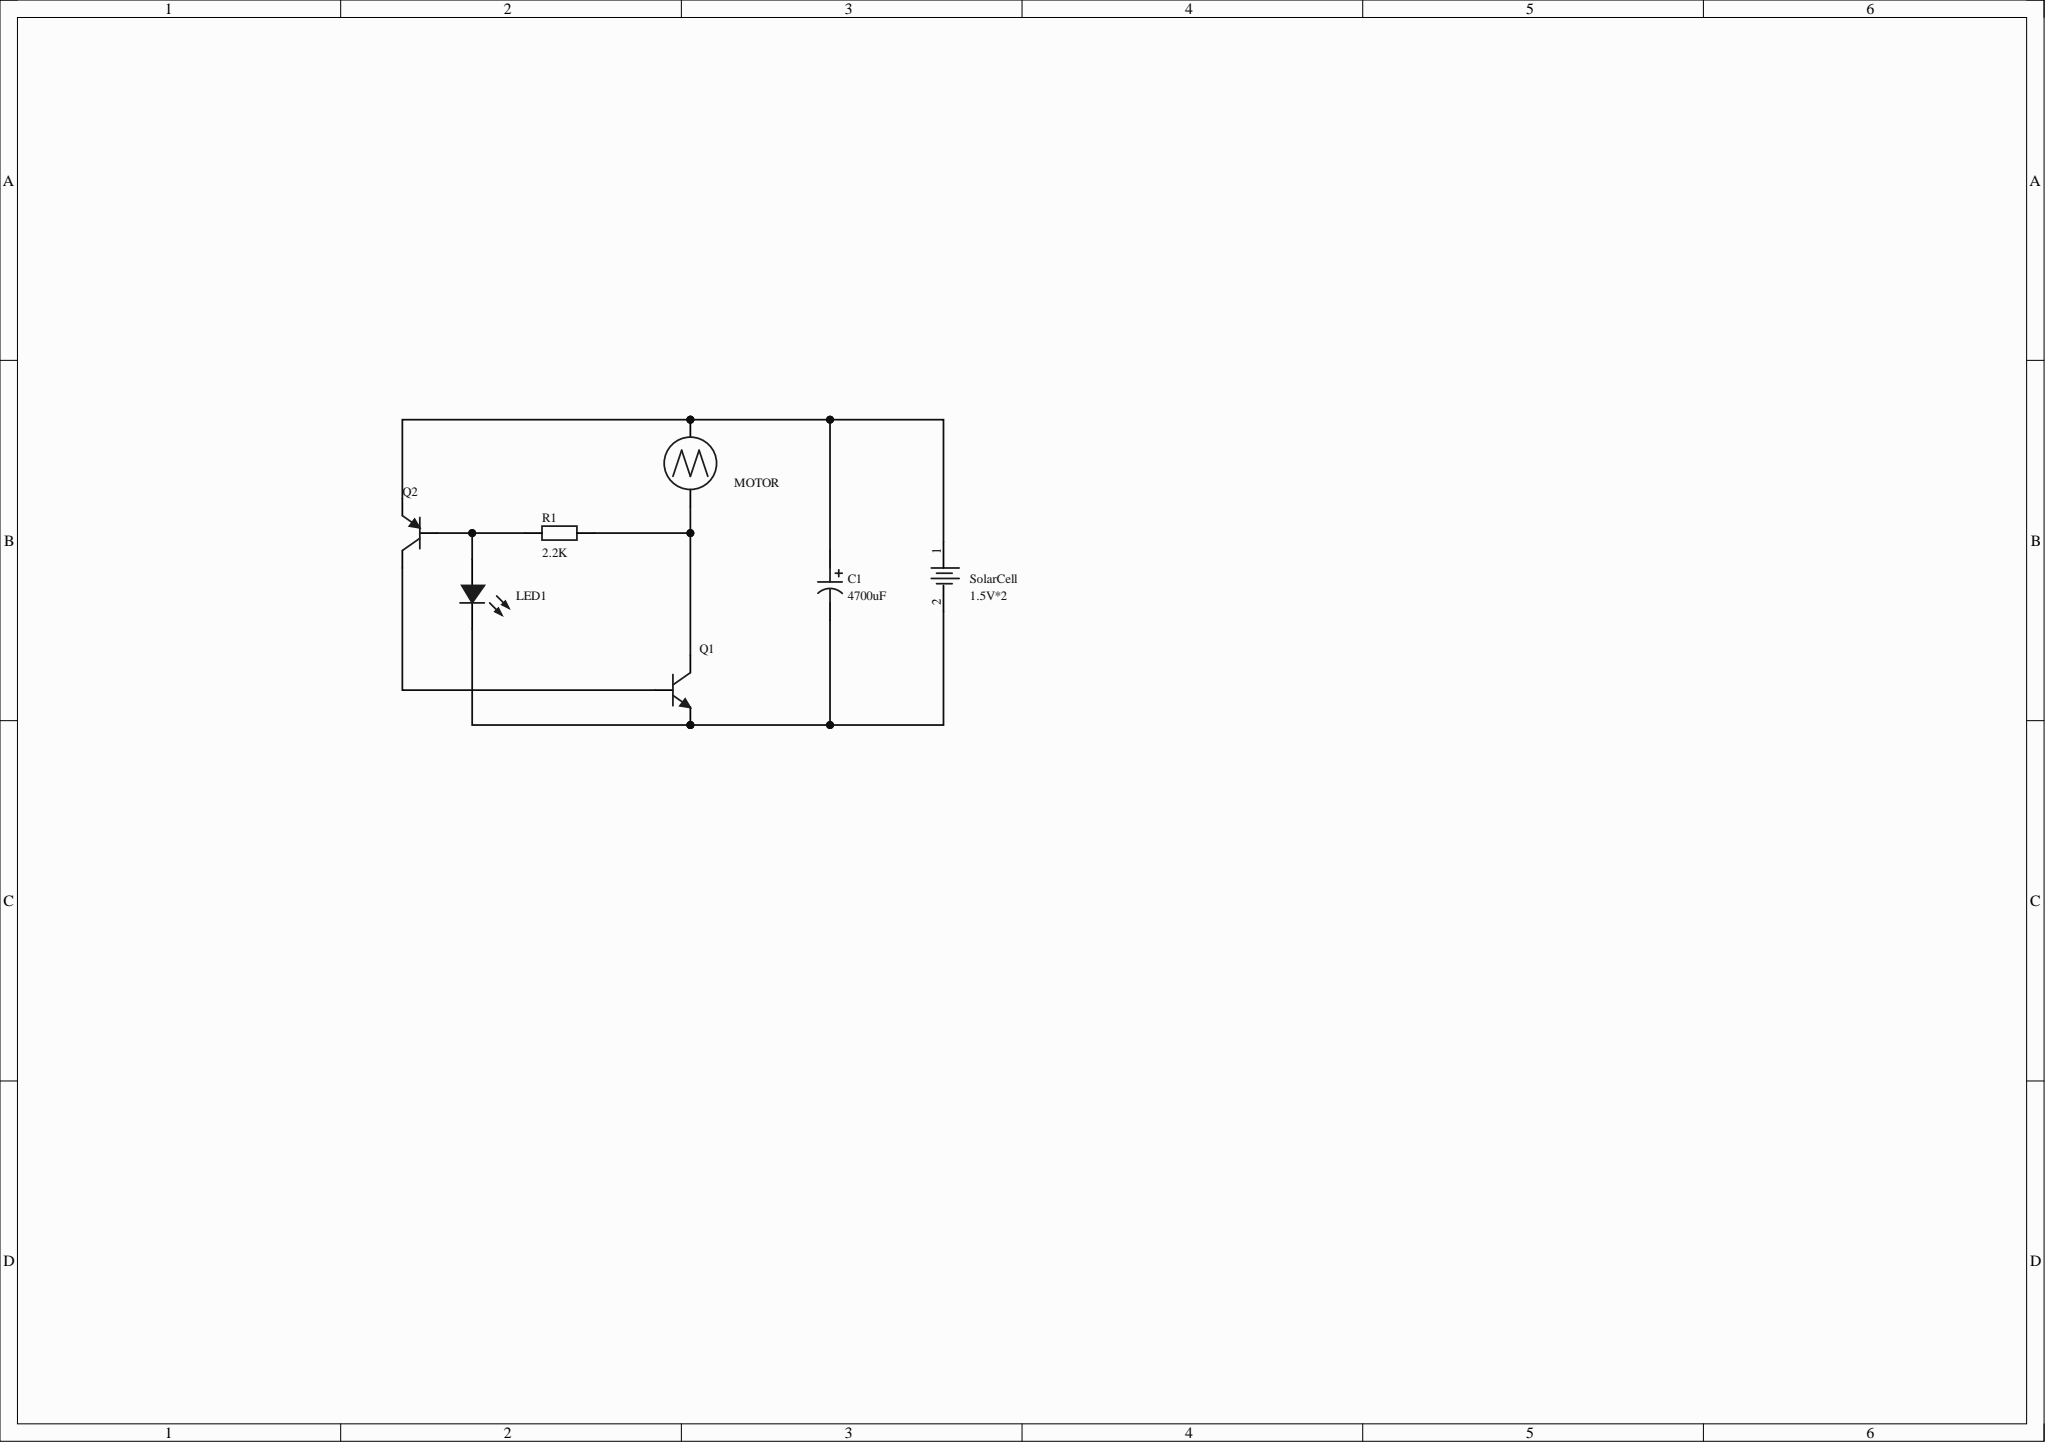Circuit board | Altium Designer | 7 parts | 5 nets
Bill of materials:
Comment,Description,Designator,Footprint,LibRef,Quantity
"4700uF","Capacitance:10uF;Tolerance:±20%;Rated voltage:50V;Ripple current:120mA@100KHz;Equivalent series resistance(ESR):1.6O;","C1","CAP-TH_BD5.0-P2.00-D0.8-FD-10UF50VC110GL","10UF50VC110GL","1"
"","","LED1","LED_0603","LED_0603-B","1"
"MOTOR_3","","MOTOR","VIBRATING-MOTOR-SMD_3P_C9900012555","MOTOR_3","1"
"","","Q1","S8050_SOT-23","S8050_SOT_NPN","1"
"","","Q2","S8550P_SOT","S8550_SOT_PNP","1"
"2.2K","","R1","R0603","Res_0603","1"
"1.5V*2","","SolarCell","BAT-TH_CR2032-2-1","CR2032-2-1","1"
Netlist (Protel format):
[
C1
CAP-TH_BD5.0-P2.00-D0.8-FD-10UF50VC110GL
4700uF



]
[
LED1
LED_0603




]
[
MOTOR
VIBRATING-MOTOR-SMD_3P_C9900012555
MOTOR_3



]
[
Q1
S8050_SOT-23




]
[
Q2
S8550P_SOT




]
[
R1
R0603
2.2K



]
[
SolarCell
BAT-TH_CR2032-2-1
1.5V*2



]
(
NetQ1_1
Q1-1
Q2-3
)
(
NetMOTOR_2
MOTOR-2
Q1-3
R1-2
)
(
NetLED1_2
LED1-2
Q2-1
R1-1
)
(
NetC1_2
C1-2
LED1-1
Q1-2
SolarCell-2
)
(
NetC1_1
C1-1
MOTOR-1
Q2-2
SolarCell-1
)